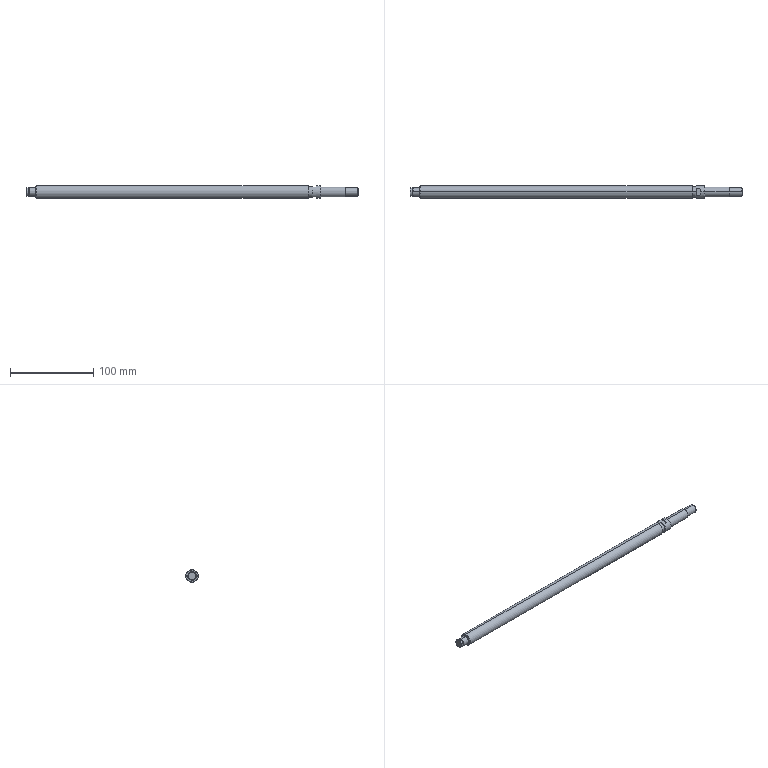Part | NX | features BREP 1 | 1 solid | 46 faces | box 400 x 15 x 15 mm | volume 65738 mm3 | cylinder 16 | plane 16 | cone 10 | torus 4 | commonest cylinder face diameters 10 x6 15 x4 9.6 x2 12 x2 12.5 x2